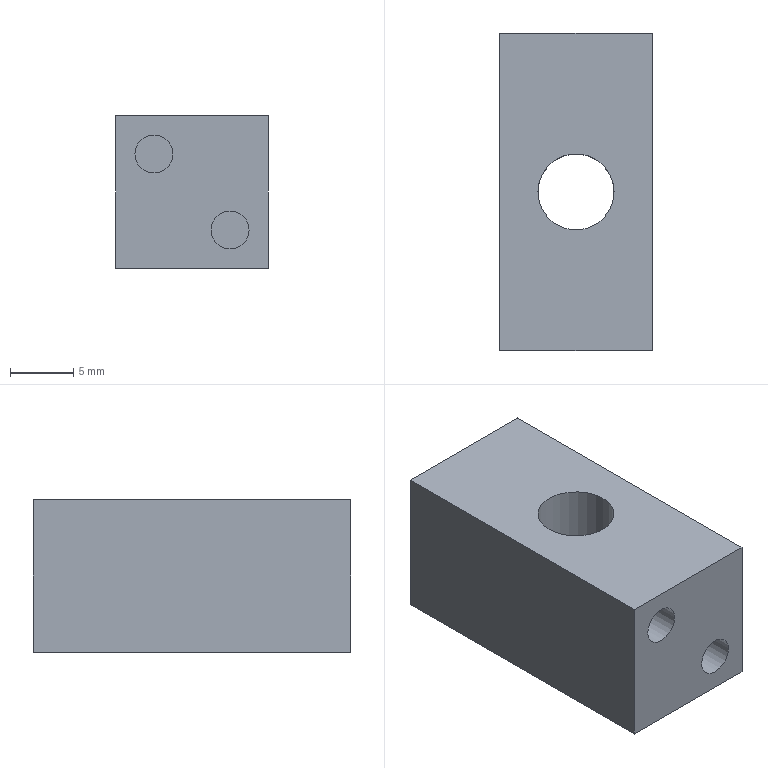Part | STEP file | 1-53.5 | 1 solid | 15 faces | box 12 x 25 x 12 mm | volume 3063 mm3 | plane 10 | cylinder 5 | commonest cylinder face diameters 3 x4 6 x1
STEP:
#1=CARTESIAN_POINT('',(0.,0.,0.));
#2=DIRECTION('',(0.,0.,1.));
#3=DIRECTION('',(1.,0.,0.));
#4=AXIS2_PLACEMENT_3D('',#1,#2,#3);
#5=CARTESIAN_POINT('',(6.,12.5,-6.));
#6=VERTEX_POINT('',#5);
#7=CARTESIAN_POINT('',(6.,12.5,6.));
#8=VERTEX_POINT('',#7);
#9=CARTESIAN_POINT('',(6.,12.5,-6.));
#10=DIRECTION('',(0.,0.,1.));
#11=VECTOR('',#10,1.);
#12=LINE('',#9,#11);
#13=CARTESIAN_POINT('',(6.,0.,0.));
#14=DIRECTION('',(1.,0.,0.));
#15=DIRECTION('',(0.,0.,1.));
#16=AXIS2_PLACEMENT_3D('',#13,#14,#15);
#17=PLANE('',#16);
#18=CARTESIAN_POINT('',(-6.,-12.5));
#19=DIRECTION('',(1.,0.));
#20=VECTOR('',#19,1.);
#21=LINE('',#18,#20);
#22=(GEOMETRIC_REPRESENTATION_CONTEXT(2)PARAMETRIC_REPRESENTATION_CONTEXT()REPRESENTATION_CONTEXT('',''));
#23=DEFINITIONAL_REPRESENTATION('',(#21),#22);
#24=PCURVE('',#17,#23);
#25=CARTESIAN_POINT('',(0.,12.5,0.));
#26=DIRECTION('',(0.,-1.,0.));
#27=DIRECTION('',(1.,0.,0.));
#28=AXIS2_PLACEMENT_3D('',#25,#26,#27);
#29=PLANE('',#28);
#30=CARTESIAN_POINT('',(6.,-6.));
#31=DIRECTION('',(0.,1.));
#32=VECTOR('',#31,1.);
#33=LINE('',#30,#32);
#34=(GEOMETRIC_REPRESENTATION_CONTEXT(2)PARAMETRIC_REPRESENTATION_CONTEXT()REPRESENTATION_CONTEXT('',''));
#35=DEFINITIONAL_REPRESENTATION('',(#33),#34);
#36=PCURVE('',#29,#35);
#37=SURFACE_CURVE('',#12,(#24,#36),.PCURVE_S1.);
#38=EDGE_CURVE('',#6,#8,#37,.T.);
#39=ORIENTED_EDGE('',*,*,#38,.T.);
#40=CARTESIAN_POINT('',(6.,-12.5,6.));
#41=VERTEX_POINT('',#40);
#42=CARTESIAN_POINT('',(6.,12.5,6.));
#43=DIRECTION('',(0.,-1.,0.));
#44=VECTOR('',#43,1.);
#45=LINE('',#42,#44);
#46=CARTESIAN_POINT('',(6.,-12.5));
#47=DIRECTION('',(0.,1.));
#48=VECTOR('',#47,1.);
#49=LINE('',#46,#48);
#50=(GEOMETRIC_REPRESENTATION_CONTEXT(2)PARAMETRIC_REPRESENTATION_CONTEXT()REPRESENTATION_CONTEXT('',''));
#51=DEFINITIONAL_REPRESENTATION('',(#49),#50);
#52=PCURVE('',#17,#51);
#53=CARTESIAN_POINT('',(0.,0.,6.));
#54=DIRECTION('',(0.,0.,1.));
#55=DIRECTION('',(-1.,0.,0.));
#56=AXIS2_PLACEMENT_3D('',#53,#54,#55);
#57=PLANE('',#56);
#58=CARTESIAN_POINT('',(-6.,-12.5));
#59=DIRECTION('',(0.,1.));
#60=VECTOR('',#59,1.);
#61=LINE('',#58,#60);
#62=(GEOMETRIC_REPRESENTATION_CONTEXT(2)PARAMETRIC_REPRESENTATION_CONTEXT()REPRESENTATION_CONTEXT('',''));
#63=DEFINITIONAL_REPRESENTATION('',(#61),#62);
#64=PCURVE('',#57,#63);
#65=SURFACE_CURVE('',#45,(#52,#64),.PCURVE_S1.);
#66=EDGE_CURVE('',#8,#41,#65,.T.);
#67=ORIENTED_EDGE('',*,*,#66,.T.);
#68=CARTESIAN_POINT('',(6.,-12.5,-6.));
#69=VERTEX_POINT('',#68);
#70=CARTESIAN_POINT('',(6.,-12.5,-6.));
#71=DIRECTION('',(0.,0.,1.));
#72=VECTOR('',#71,1.);
#73=LINE('',#70,#72);
#74=CARTESIAN_POINT('',(-6.,12.5));
#75=DIRECTION('',(1.,0.));
#76=VECTOR('',#75,1.);
#77=LINE('',#74,#76);
#78=(GEOMETRIC_REPRESENTATION_CONTEXT(2)PARAMETRIC_REPRESENTATION_CONTEXT()REPRESENTATION_CONTEXT('',''));
#79=DEFINITIONAL_REPRESENTATION('',(#77),#78);
#80=PCURVE('',#17,#79);
#81=CARTESIAN_POINT('',(0.,-12.5,0.));
#82=DIRECTION('',(0.,-1.,0.));
#83=DIRECTION('',(1.,0.,0.));
#84=AXIS2_PLACEMENT_3D('',#81,#82,#83);
#85=PLANE('',#84);
#86=CARTESIAN_POINT('',(6.,-6.));
#87=DIRECTION('',(0.,1.));
#88=VECTOR('',#87,1.);
#89=LINE('',#86,#88);
#90=(GEOMETRIC_REPRESENTATION_CONTEXT(2)PARAMETRIC_REPRESENTATION_CONTEXT()REPRESENTATION_CONTEXT('',''));
#91=DEFINITIONAL_REPRESENTATION('',(#89),#90);
#92=PCURVE('',#85,#91);
#93=SURFACE_CURVE('',#73,(#80,#92),.PCURVE_S1.);
#94=EDGE_CURVE('',#69,#41,#93,.T.);
#95=ORIENTED_EDGE('',*,*,#94,.F.);
#96=CARTESIAN_POINT('',(6.,12.5,-6.));
#97=DIRECTION('',(0.,-1.,0.));
#98=VECTOR('',#97,1.);
#99=LINE('',#96,#98);
#100=CARTESIAN_POINT('',(-6.,-12.5));
#101=DIRECTION('',(0.,1.));
#102=VECTOR('',#101,1.);
#103=LINE('',#100,#102);
#104=(GEOMETRIC_REPRESENTATION_CONTEXT(2)PARAMETRIC_REPRESENTATION_CONTEXT()REPRESENTATION_CONTEXT('',''));
#105=DEFINITIONAL_REPRESENTATION('',(#103),#104);
#106=PCURVE('',#17,#105);
#107=CARTESIAN_POINT('',(0.,0.,-6.));
#108=DIRECTION('',(0.,0.,-1.));
#109=DIRECTION('',(1.,0.,0.));
#110=AXIS2_PLACEMENT_3D('',#107,#108,#109);
#111=PLANE('',#110);
#112=CARTESIAN_POINT('',(6.,-12.5));
#113=DIRECTION('',(0.,1.));
#114=VECTOR('',#113,1.);
#115=LINE('',#112,#114);
#116=(GEOMETRIC_REPRESENTATION_CONTEXT(2)PARAMETRIC_REPRESENTATION_CONTEXT()REPRESENTATION_CONTEXT('',''));
#117=DEFINITIONAL_REPRESENTATION('',(#115),#116);
#118=PCURVE('',#111,#117);
#119=SURFACE_CURVE('',#99,(#106,#118),.PCURVE_S1.);
#120=EDGE_CURVE('',#6,#69,#119,.T.);
#121=ORIENTED_EDGE('',*,*,#120,.F.);
#122=EDGE_LOOP('',(#39,#67,#95,#121));
#123=FACE_BOUND('',#122,.T.);
#124=ADVANCED_FACE('',(#123),#17,.T.);
#125=CARTESIAN_POINT('',(-6.,12.5,6.));
#126=VERTEX_POINT('',#125);
#127=CARTESIAN_POINT('',(-6.,12.5,-6.));
#128=VERTEX_POINT('',#127);
#129=CARTESIAN_POINT('',(-6.,12.5,6.));
#130=DIRECTION('',(0.,0.,-1.));
#131=VECTOR('',#130,1.);
#132=LINE('',#129,#131);
#133=CARTESIAN_POINT('',(-6.,0.,0.));
#134=DIRECTION('',(-1.,0.,0.));
#135=DIRECTION('',(0.,0.,-1.));
#136=AXIS2_PLACEMENT_3D('',#133,#134,#135);
#137=PLANE('',#136);
#138=CARTESIAN_POINT('',(-6.,-12.5));
#139=DIRECTION('',(1.,0.));
#140=VECTOR('',#139,1.);
#141=LINE('',#138,#140);
#142=(GEOMETRIC_REPRESENTATION_CONTEXT(2)PARAMETRIC_REPRESENTATION_CONTEXT()REPRESENTATION_CONTEXT('',''));
#143=DEFINITIONAL_REPRESENTATION('',(#141),#142);
#144=PCURVE('',#137,#143);
#145=CARTESIAN_POINT('',(-6.,6.));
#146=DIRECTION('',(0.,-1.));
#147=VECTOR('',#146,1.);
#148=LINE('',#145,#147);
#149=(GEOMETRIC_REPRESENTATION_CONTEXT(2)PARAMETRIC_REPRESENTATION_CONTEXT()REPRESENTATION_CONTEXT('',''));
#150=DEFINITIONAL_REPRESENTATION('',(#148),#149);
#151=PCURVE('',#29,#150);
#152=SURFACE_CURVE('',#132,(#144,#151),.PCURVE_S1.);
#153=EDGE_CURVE('',#126,#128,#152,.T.);
#154=ORIENTED_EDGE('',*,*,#153,.T.);
#155=CARTESIAN_POINT('',(-6.,-12.5,-6.));
#156=VERTEX_POINT('',#155);
#157=CARTESIAN_POINT('',(-6.,12.5,-6.));
#158=DIRECTION('',(0.,-1.,0.));
#159=VECTOR('',#158,1.);
#160=LINE('',#157,#159);
#161=CARTESIAN_POINT('',(6.,-12.5));
#162=DIRECTION('',(0.,1.));
#163=VECTOR('',#162,1.);
#164=LINE('',#161,#163);
#165=(GEOMETRIC_REPRESENTATION_CONTEXT(2)PARAMETRIC_REPRESENTATION_CONTEXT()REPRESENTATION_CONTEXT('',''));
#166=DEFINITIONAL_REPRESENTATION('',(#164),#165);
#167=PCURVE('',#137,#166);
#168=CARTESIAN_POINT('',(-6.,-12.5));
#169=DIRECTION('',(0.,1.));
#170=VECTOR('',#169,1.);
#171=LINE('',#168,#170);
#172=(GEOMETRIC_REPRESENTATION_CONTEXT(2)PARAMETRIC_REPRESENTATION_CONTEXT()REPRESENTATION_CONTEXT('',''));
#173=DEFINITIONAL_REPRESENTATION('',(#171),#172);
#174=PCURVE('',#111,#173);
#175=SURFACE_CURVE('',#160,(#167,#174),.PCURVE_S1.);
#176=EDGE_CURVE('',#128,#156,#175,.T.);
#177=ORIENTED_EDGE('',*,*,#176,.T.);
#178=CARTESIAN_POINT('',(-6.,-12.5,6.));
#179=VERTEX_POINT('',#178);
#180=CARTESIAN_POINT('',(-6.,-12.5,6.));
#181=DIRECTION('',(0.,0.,-1.));
#182=VECTOR('',#181,1.);
#183=LINE('',#180,#182);
#184=CARTESIAN_POINT('',(-6.,12.5));
#185=DIRECTION('',(1.,0.));
#186=VECTOR('',#185,1.);
#187=LINE('',#184,#186);
#188=(GEOMETRIC_REPRESENTATION_CONTEXT(2)PARAMETRIC_REPRESENTATION_CONTEXT()REPRESENTATION_CONTEXT('',''));
#189=DEFINITIONAL_REPRESENTATION('',(#187),#188);
#190=PCURVE('',#137,#189);
#191=CARTESIAN_POINT('',(-6.,6.));
#192=DIRECTION('',(0.,-1.));
#193=VECTOR('',#192,1.);
#194=LINE('',#191,#193);
#195=(GEOMETRIC_REPRESENTATION_CONTEXT(2)PARAMETRIC_REPRESENTATION_CONTEXT()REPRESENTATION_CONTEXT('',''));
#196=DEFINITIONAL_REPRESENTATION('',(#194),#195);
#197=PCURVE('',#85,#196);
#198=SURFACE_CURVE('',#183,(#190,#197),.PCURVE_S1.);
#199=EDGE_CURVE('',#179,#156,#198,.T.);
#200=ORIENTED_EDGE('',*,*,#199,.F.);
#201=CARTESIAN_POINT('',(-6.,12.5,6.));
#202=DIRECTION('',(0.,-1.,0.));
#203=VECTOR('',#202,1.);
#204=LINE('',#201,#203);
#205=CARTESIAN_POINT('',(-6.,-12.5));
#206=DIRECTION('',(0.,1.));
#207=VECTOR('',#206,1.);
#208=LINE('',#205,#207);
#209=(GEOMETRIC_REPRESENTATION_CONTEXT(2)PARAMETRIC_REPRESENTATION_CONTEXT()REPRESENTATION_CONTEXT('',''));
#210=DEFINITIONAL_REPRESENTATION('',(#208),#209);
#211=PCURVE('',#137,#210);
#212=CARTESIAN_POINT('',(6.,-12.5));
#213=DIRECTION('',(0.,1.));
#214=VECTOR('',#213,1.);
#215=LINE('',#212,#214);
#216=(GEOMETRIC_REPRESENTATION_CONTEXT(2)PARAMETRIC_REPRESENTATION_CONTEXT()REPRESENTATION_CONTEXT('',''));
#217=DEFINITIONAL_REPRESENTATION('',(#215),#216);
#218=PCURVE('',#57,#217);
#219=SURFACE_CURVE('',#204,(#211,#218),.PCURVE_S1.);
#220=EDGE_CURVE('',#126,#179,#219,.T.);
#221=ORIENTED_EDGE('',*,*,#220,.F.);
#222=EDGE_LOOP('',(#154,#177,#200,#221));
#223=FACE_BOUND('',#222,.T.);
#224=ADVANCED_FACE('',(#223),#137,.T.);
#225=CARTESIAN_POINT('',(-6.,-12.5,-6.));
#226=DIRECTION('',(1.,0.,0.));
#227=VECTOR('',#226,1.);
#228=LINE('',#225,#227);
#229=CARTESIAN_POINT('',(-6.,-6.));
#230=DIRECTION('',(1.,0.));
#231=VECTOR('',#230,1.);
#232=LINE('',#229,#231);
#233=(GEOMETRIC_REPRESENTATION_CONTEXT(2)PARAMETRIC_REPRESENTATION_CONTEXT()REPRESENTATION_CONTEXT('',''));
#234=DEFINITIONAL_REPRESENTATION('',(#232),#233);
#235=PCURVE('',#85,#234);
#236=CARTESIAN_POINT('',(-6.,12.5));
#237=DIRECTION('',(1.,0.));
#238=VECTOR('',#237,1.);
#239=LINE('',#236,#238);
#240=(GEOMETRIC_REPRESENTATION_CONTEXT(2)PARAMETRIC_REPRESENTATION_CONTEXT()REPRESENTATION_CONTEXT('',''));
#241=DEFINITIONAL_REPRESENTATION('',(#239),#240);
#242=PCURVE('',#111,#241);
#243=SURFACE_CURVE('',#228,(#235,#242),.PCURVE_S1.);
#244=EDGE_CURVE('',#156,#69,#243,.T.);
#245=ORIENTED_EDGE('',*,*,#244,.T.);
#246=ORIENTED_EDGE('',*,*,#94,.T.);
#247=CARTESIAN_POINT('',(6.,-12.5,6.));
#248=DIRECTION('',(-1.,0.,0.));
#249=VECTOR('',#248,1.);
#250=LINE('',#247,#249);
#251=CARTESIAN_POINT('',(6.,6.));
#252=DIRECTION('',(-1.,0.));
#253=VECTOR('',#252,1.);
#254=LINE('',#251,#253);
#255=(GEOMETRIC_REPRESENTATION_CONTEXT(2)PARAMETRIC_REPRESENTATION_CONTEXT()REPRESENTATION_CONTEXT('',''));
#256=DEFINITIONAL_REPRESENTATION('',(#254),#255);
#257=PCURVE('',#85,#256);
#258=CARTESIAN_POINT('',(-6.,12.5));
#259=DIRECTION('',(1.,0.));
#260=VECTOR('',#259,1.);
#261=LINE('',#258,#260);
#262=(GEOMETRIC_REPRESENTATION_CONTEXT(2)PARAMETRIC_REPRESENTATION_CONTEXT()REPRESENTATION_CONTEXT('',''));
#263=DEFINITIONAL_REPRESENTATION('',(#261),#262);
#264=PCURVE('',#57,#263);
#265=SURFACE_CURVE('',#250,(#257,#264),.PCURVE_S1.);
#266=EDGE_CURVE('',#41,#179,#265,.T.);
#267=ORIENTED_EDGE('',*,*,#266,.T.);
#268=ORIENTED_EDGE('',*,*,#199,.T.);
#269=EDGE_LOOP('',(#245,#246,#267,#268));
#270=FACE_BOUND('',#269,.T.);
#271=CARTESIAN_POINT('',(-1.5,-12.5,3.));
#272=VERTEX_POINT('',#271);
#273=CARTESIAN_POINT('',(-3.,-12.5,3.));
#274=DIRECTION('',(0.,-1.,0.));
#275=DIRECTION('',(1.,0.,0.));
#276=AXIS2_PLACEMENT_3D('',#273,#274,#275);
#277=CIRCLE('',#276,1.5);
#278=CARTESIAN_POINT('',(-3.,3.));
#279=DIRECTION('',(1.,0.));
#280=AXIS2_PLACEMENT_2D('',#278,#279);
#281=CIRCLE('',#280,1.5);
#282=(GEOMETRIC_REPRESENTATION_CONTEXT(2)PARAMETRIC_REPRESENTATION_CONTEXT()REPRESENTATION_CONTEXT('',''));
#283=DEFINITIONAL_REPRESENTATION('',(#281),#282);
#284=PCURVE('',#85,#283);
#285=CARTESIAN_POINT('',(-3.,-12.5,3.));
#286=DIRECTION('',(0.,1.,0.));
#287=DIRECTION('',(1.,0.,0.));
#288=AXIS2_PLACEMENT_3D('',#285,#286,#287);
#289=CYLINDRICAL_SURFACE('',#288,1.5);
#290=CARTESIAN_POINT('',(6.283,0.));
#291=DIRECTION('',(-1.,0.));
#292=VECTOR('',#291,1.);
#293=LINE('',#290,#292);
#294=(GEOMETRIC_REPRESENTATION_CONTEXT(2)PARAMETRIC_REPRESENTATION_CONTEXT()REPRESENTATION_CONTEXT('',''));
#295=DEFINITIONAL_REPRESENTATION('',(#293),#294);
#296=PCURVE('',#289,#295);
#297=SURFACE_CURVE('',#277,(#284,#296),.PCURVE_S1.);
#298=EDGE_CURVE('',#272,#272,#297,.T.);
#299=ORIENTED_EDGE('',*,*,#298,.F.);
#300=EDGE_LOOP('',(#299));
#301=FACE_BOUND('',#300,.T.);
#302=CARTESIAN_POINT('',(4.5,-12.5,-3.));
#303=VERTEX_POINT('',#302);
#304=CARTESIAN_POINT('',(3.,-12.5,-3.));
#305=DIRECTION('',(0.,-1.,0.));
#306=DIRECTION('',(1.,0.,0.));
#307=AXIS2_PLACEMENT_3D('',#304,#305,#306);
#308=CIRCLE('',#307,1.5);
#309=CARTESIAN_POINT('',(3.,-3.));
#310=DIRECTION('',(1.,0.));
#311=AXIS2_PLACEMENT_2D('',#309,#310);
#312=CIRCLE('',#311,1.5);
#313=(GEOMETRIC_REPRESENTATION_CONTEXT(2)PARAMETRIC_REPRESENTATION_CONTEXT()REPRESENTATION_CONTEXT('',''));
#314=DEFINITIONAL_REPRESENTATION('',(#312),#313);
#315=PCURVE('',#85,#314);
#316=CARTESIAN_POINT('',(3.,-12.5,-3.));
#317=DIRECTION('',(0.,1.,0.));
#318=DIRECTION('',(1.,0.,0.));
#319=AXIS2_PLACEMENT_3D('',#316,#317,#318);
#320=CYLINDRICAL_SURFACE('',#319,1.5);
#321=CARTESIAN_POINT('',(6.283,0.));
#322=DIRECTION('',(-1.,0.));
#323=VECTOR('',#322,1.);
#324=LINE('',#321,#323);
#325=(GEOMETRIC_REPRESENTATION_CONTEXT(2)PARAMETRIC_REPRESENTATION_CONTEXT()REPRESENTATION_CONTEXT('',''));
#326=DEFINITIONAL_REPRESENTATION('',(#324),#325);
#327=PCURVE('',#320,#326);
#328=SURFACE_CURVE('',#308,(#315,#327),.PCURVE_S1.);
#329=EDGE_CURVE('',#303,#303,#328,.T.);
#330=ORIENTED_EDGE('',*,*,#329,.F.);
#331=EDGE_LOOP('',(#330));
#332=FACE_BOUND('',#331,.T.);
#333=ADVANCED_FACE('',(#270,#301,#332),#85,.T.);
#334=CARTESIAN_POINT('',(-1.5,-5.5,3.));
#335=VERTEX_POINT('',#334);
#336=CARTESIAN_POINT('',(-1.5,-12.5,3.));
#337=DIRECTION('',(0.,1.,0.));
#338=VECTOR('',#337,1.);
#339=LINE('',#336,#338);
#340=CARTESIAN_POINT('',(6.283,0.));
#341=DIRECTION('',(0.,1.));
#342=VECTOR('',#341,1.);
#343=LINE('',#340,#342);
#344=(GEOMETRIC_REPRESENTATION_CONTEXT(2)PARAMETRIC_REPRESENTATION_CONTEXT()REPRESENTATION_CONTEXT('',''));
#345=DEFINITIONAL_REPRESENTATION('',(#343),#344);
#346=PCURVE('',#289,#345);
#347=CARTESIAN_POINT('',(0.,0.));
#348=DIRECTION('',(0.,1.));
#349=VECTOR('',#348,1.);
#350=LINE('',#347,#349);
#351=(GEOMETRIC_REPRESENTATION_CONTEXT(2)PARAMETRIC_REPRESENTATION_CONTEXT()REPRESENTATION_CONTEXT('',''));
#352=DEFINITIONAL_REPRESENTATION('',(#350),#351);
#353=PCURVE('',#289,#352);
#354=SEAM_CURVE('',#339,(#346,#353),.PCURVE_S1.);
#355=EDGE_CURVE('',#272,#335,#354,.T.);
#356=ORIENTED_EDGE('',*,*,#355,.T.);
#357=CARTESIAN_POINT('',(-3.,-5.5,3.));
#358=DIRECTION('',(0.,-1.,0.));
#359=DIRECTION('',(1.,0.,0.));
#360=AXIS2_PLACEMENT_3D('',#357,#358,#359);
#361=CIRCLE('',#360,1.5);
#362=CARTESIAN_POINT('',(6.283,7.));
#363=DIRECTION('',(-1.,0.));
#364=VECTOR('',#363,1.);
#365=LINE('',#362,#364);
#366=(GEOMETRIC_REPRESENTATION_CONTEXT(2)PARAMETRIC_REPRESENTATION_CONTEXT()REPRESENTATION_CONTEXT('',''));
#367=DEFINITIONAL_REPRESENTATION('',(#365),#366);
#368=PCURVE('',#289,#367);
#369=CARTESIAN_POINT('',(-3.402,-5.5,3.));
#370=DIRECTION('',(0.,-1.,0.));
#371=DIRECTION('',(1.,0.,0.));
#372=AXIS2_PLACEMENT_3D('',#369,#370,#371);
#373=PLANE('',#372);
#374=CARTESIAN_POINT('',(0.4019,0.));
#375=DIRECTION('',(1.,0.));
#376=AXIS2_PLACEMENT_2D('',#374,#375);
#377=CIRCLE('',#376,1.5);
#378=(GEOMETRIC_REPRESENTATION_CONTEXT(2)PARAMETRIC_REPRESENTATION_CONTEXT()REPRESENTATION_CONTEXT('',''));
#379=DEFINITIONAL_REPRESENTATION('',(#377),#378);
#380=PCURVE('',#373,#379);
#381=SURFACE_CURVE('',#361,(#368,#380),.PCURVE_S1.);
#382=EDGE_CURVE('',#335,#335,#381,.T.);
#383=ORIENTED_EDGE('',*,*,#382,.T.);
#384=ORIENTED_EDGE('',*,*,#355,.F.);
#385=ORIENTED_EDGE('',*,*,#298,.F.);
#386=EDGE_LOOP('',(#356,#383,#384,#385));
#387=FACE_BOUND('',#386,.F.);
#388=ADVANCED_FACE('',(#387),#289,.F.);
#389=CARTESIAN_POINT('',(4.5,-5.5,-3.));
#390=VERTEX_POINT('',#389);
#391=CARTESIAN_POINT('',(4.5,-12.5,-3.));
#392=DIRECTION('',(0.,1.,0.));
#393=VECTOR('',#392,1.);
#394=LINE('',#391,#393);
#395=CARTESIAN_POINT('',(6.283,0.));
#396=DIRECTION('',(0.,1.));
#397=VECTOR('',#396,1.);
#398=LINE('',#395,#397);
#399=(GEOMETRIC_REPRESENTATION_CONTEXT(2)PARAMETRIC_REPRESENTATION_CONTEXT()REPRESENTATION_CONTEXT('',''));
#400=DEFINITIONAL_REPRESENTATION('',(#398),#399);
#401=PCURVE('',#320,#400);
#402=CARTESIAN_POINT('',(0.,0.));
#403=DIRECTION('',(0.,1.));
#404=VECTOR('',#403,1.);
#405=LINE('',#402,#404);
#406=(GEOMETRIC_REPRESENTATION_CONTEXT(2)PARAMETRIC_REPRESENTATION_CONTEXT()REPRESENTATION_CONTEXT('',''));
#407=DEFINITIONAL_REPRESENTATION('',(#405),#406);
#408=PCURVE('',#320,#407);
#409=SEAM_CURVE('',#394,(#401,#408),.PCURVE_S1.);
#410=EDGE_CURVE('',#303,#390,#409,.T.);
#411=ORIENTED_EDGE('',*,*,#410,.T.);
#412=CARTESIAN_POINT('',(3.,-5.5,-3.));
#413=DIRECTION('',(0.,-1.,0.));
#414=DIRECTION('',(1.,0.,0.));
#415=AXIS2_PLACEMENT_3D('',#412,#413,#414);
#416=CIRCLE('',#415,1.5);
#417=CARTESIAN_POINT('',(6.283,7.));
#418=DIRECTION('',(-1.,0.));
#419=VECTOR('',#418,1.);
#420=LINE('',#417,#419);
#421=(GEOMETRIC_REPRESENTATION_CONTEXT(2)PARAMETRIC_REPRESENTATION_CONTEXT()REPRESENTATION_CONTEXT('',''));
#422=DEFINITIONAL_REPRESENTATION('',(#420),#421);
#423=PCURVE('',#320,#422);
#424=CARTESIAN_POINT('',(2.598,-5.5,-3.));
#425=DIRECTION('',(0.,-1.,0.));
#426=DIRECTION('',(1.,0.,0.));
#427=AXIS2_PLACEMENT_3D('',#424,#425,#426);
#428=PLANE('',#427);
#429=CARTESIAN_POINT('',(0.4019,0.));
#430=DIRECTION('',(1.,0.));
#431=AXIS2_PLACEMENT_2D('',#429,#430);
#432=CIRCLE('',#431,1.5);
#433=(GEOMETRIC_REPRESENTATION_CONTEXT(2)PARAMETRIC_REPRESENTATION_CONTEXT()REPRESENTATION_CONTEXT('',''));
#434=DEFINITIONAL_REPRESENTATION('',(#432),#433);
#435=PCURVE('',#428,#434);
#436=SURFACE_CURVE('',#416,(#423,#435),.PCURVE_S1.);
#437=EDGE_CURVE('',#390,#390,#436,.T.);
#438=ORIENTED_EDGE('',*,*,#437,.T.);
#439=ORIENTED_EDGE('',*,*,#410,.F.);
#440=ORIENTED_EDGE('',*,*,#329,.F.);
#441=EDGE_LOOP('',(#411,#438,#439,#440));
#442=FACE_BOUND('',#441,.F.);
#443=ADVANCED_FACE('',(#442),#320,.F.);
#444=ORIENTED_EDGE('',*,*,#382,.T.);
#445=EDGE_LOOP('',(#444));
#446=FACE_BOUND('',#445,.T.);
#447=ADVANCED_FACE('',(#446),#373,.T.);
#448=ORIENTED_EDGE('',*,*,#437,.T.);
#449=EDGE_LOOP('',(#448));
#450=FACE_BOUND('',#449,.T.);
#451=ADVANCED_FACE('',(#450),#428,.T.);
#452=CARTESIAN_POINT('',(-6.,12.5,-6.));
#453=DIRECTION('',(1.,0.,0.));
#454=VECTOR('',#453,1.);
#455=LINE('',#452,#454);
#456=CARTESIAN_POINT('',(-6.,-12.5));
#457=DIRECTION('',(1.,0.));
#458=VECTOR('',#457,1.);
#459=LINE('',#456,#458);
#460=(GEOMETRIC_REPRESENTATION_CONTEXT(2)PARAMETRIC_REPRESENTATION_CONTEXT()REPRESENTATION_CONTEXT('',''));
#461=DEFINITIONAL_REPRESENTATION('',(#459),#460);
#462=PCURVE('',#111,#461);
#463=CARTESIAN_POINT('',(-6.,-6.));
#464=DIRECTION('',(1.,0.));
#465=VECTOR('',#464,1.);
#466=LINE('',#463,#465);
#467=(GEOMETRIC_REPRESENTATION_CONTEXT(2)PARAMETRIC_REPRESENTATION_CONTEXT()REPRESENTATION_CONTEXT('',''));
#468=DEFINITIONAL_REPRESENTATION('',(#466),#467);
#469=PCURVE('',#29,#468);
#470=SURFACE_CURVE('',#455,(#462,#469),.PCURVE_S1.);
#471=EDGE_CURVE('',#128,#6,#470,.T.);
#472=ORIENTED_EDGE('',*,*,#471,.T.);
#473=ORIENTED_EDGE('',*,*,#120,.T.);
#474=ORIENTED_EDGE('',*,*,#244,.F.);
#475=ORIENTED_EDGE('',*,*,#176,.F.);
#476=EDGE_LOOP('',(#472,#473,#474,#475));
#477=FACE_BOUND('',#476,.T.);
#478=CARTESIAN_POINT('',(3.,0.,-6.));
#479=VERTEX_POINT('',#478);
#480=CARTESIAN_POINT('',(0.,0.,-6.));
#481=DIRECTION('',(0.,0.,1.));
#482=DIRECTION('',(1.,0.,0.));
#483=AXIS2_PLACEMENT_3D('',#480,#481,#482);
#484=CIRCLE('',#483,3.);
#485=CARTESIAN_POINT('',(3.,0.));
#486=CARTESIAN_POINT('',(3.,-5.196));
#487=CARTESIAN_POINT('',(-1.5,-2.598));
#488=CARTESIAN_POINT('',(-6.,0.));
#489=CARTESIAN_POINT('',(-1.5,2.598));
#490=CARTESIAN_POINT('',(3.,5.196));
#491=CARTESIAN_POINT('',(3.,0.));
#492=(BOUNDED_CURVE()B_SPLINE_CURVE(2,(#485,#486,#487,#488,#489,#490,#491),.UNSPECIFIED.,.T.,.F.)B_SPLINE_CURVE_WITH_KNOTS((1,2,2,2,2,1),(-2.094,0.,2.094,4.189,6.283,8.378),.UNSPECIFIED.)CURVE()GEOMETRIC_REPRESENTATION_ITEM()RATIONAL_B_SPLINE_CURVE((1.,0.5,1.,0.5,1.,0.5,1.))REPRESENTATION_ITEM(''));
#493=(GEOMETRIC_REPRESENTATION_CONTEXT(2)PARAMETRIC_REPRESENTATION_CONTEXT()REPRESENTATION_CONTEXT('',''));
#494=DEFINITIONAL_REPRESENTATION('',(#492),#493);
#495=PCURVE('',#111,#494);
#496=CARTESIAN_POINT('',(0.,0.,6.));
#497=DIRECTION('',(0.,0.,-1.));
#498=DIRECTION('',(1.,0.,0.));
#499=AXIS2_PLACEMENT_3D('',#496,#497,#498);
#500=CYLINDRICAL_SURFACE('',#499,3.);
#501=CARTESIAN_POINT('',(6.283,12.));
#502=DIRECTION('',(-1.,0.));
#503=VECTOR('',#502,1.);
#504=LINE('',#501,#503);
#505=(GEOMETRIC_REPRESENTATION_CONTEXT(2)PARAMETRIC_REPRESENTATION_CONTEXT()REPRESENTATION_CONTEXT('',''));
#506=DEFINITIONAL_REPRESENTATION('',(#504),#505);
#507=PCURVE('',#500,#506);
#508=SURFACE_CURVE('',#484,(#495,#507),.PCURVE_S1.);
#509=EDGE_CURVE('',#479,#479,#508,.T.);
#510=ORIENTED_EDGE('',*,*,#509,.T.);
#511=EDGE_LOOP('',(#510));
#512=FACE_BOUND('',#511,.T.);
#513=ADVANCED_FACE('',(#477,#512),#111,.T.);
#514=CARTESIAN_POINT('',(6.,12.5,6.));
#515=DIRECTION('',(-1.,0.,0.));
#516=VECTOR('',#515,1.);
#517=LINE('',#514,#516);
#518=CARTESIAN_POINT('',(-6.,-12.5));
#519=DIRECTION('',(1.,0.));
#520=VECTOR('',#519,1.);
#521=LINE('',#518,#520);
#522=(GEOMETRIC_REPRESENTATION_CONTEXT(2)PARAMETRIC_REPRESENTATION_CONTEXT()REPRESENTATION_CONTEXT('',''));
#523=DEFINITIONAL_REPRESENTATION('',(#521),#522);
#524=PCURVE('',#57,#523);
#525=CARTESIAN_POINT('',(6.,6.));
#526=DIRECTION('',(-1.,0.));
#527=VECTOR('',#526,1.);
#528=LINE('',#525,#527);
#529=(GEOMETRIC_REPRESENTATION_CONTEXT(2)PARAMETRIC_REPRESENTATION_CONTEXT()REPRESENTATION_CONTEXT('',''));
#530=DEFINITIONAL_REPRESENTATION('',(#528),#529);
#531=PCURVE('',#29,#530);
#532=SURFACE_CURVE('',#517,(#524,#531),.PCURVE_S1.);
#533=EDGE_CURVE('',#8,#126,#532,.T.);
#534=ORIENTED_EDGE('',*,*,#533,.T.);
#535=ORIENTED_EDGE('',*,*,#220,.T.);
#536=ORIENTED_EDGE('',*,*,#266,.F.);
#537=ORIENTED_EDGE('',*,*,#66,.F.);
#538=EDGE_LOOP('',(#534,#535,#536,#537));
#539=FACE_BOUND('',#538,.T.);
#540=CARTESIAN_POINT('',(3.,0.,6.));
#541=VERTEX_POINT('',#540);
#542=CARTESIAN_POINT('',(0.,0.,6.));
#543=DIRECTION('',(0.,0.,1.));
#544=DIRECTION('',(1.,0.,0.));
#545=AXIS2_PLACEMENT_3D('',#542,#543,#544);
#546=CIRCLE('',#545,3.);
#547=CARTESIAN_POINT('',(0.,0.));
#548=DIRECTION('',(-1.,0.));
#549=AXIS2_PLACEMENT_2D('',#547,#548);
#550=CIRCLE('',#549,3.);
#551=(GEOMETRIC_REPRESENTATION_CONTEXT(2)PARAMETRIC_REPRESENTATION_CONTEXT()REPRESENTATION_CONTEXT('',''));
#552=DEFINITIONAL_REPRESENTATION('',(#550),#551);
#553=PCURVE('',#57,#552);
#554=CARTESIAN_POINT('',(6.283,0.));
#555=DIRECTION('',(-1.,0.));
#556=VECTOR('',#555,1.);
#557=LINE('',#554,#556);
#558=(GEOMETRIC_REPRESENTATION_CONTEXT(2)PARAMETRIC_REPRESENTATION_CONTEXT()REPRESENTATION_CONTEXT('',''));
#559=DEFINITIONAL_REPRESENTATION('',(#557),#558);
#560=PCURVE('',#500,#559);
#561=SURFACE_CURVE('',#546,(#553,#560),.PCURVE_S1.);
#562=EDGE_CURVE('',#541,#541,#561,.T.);
#563=ORIENTED_EDGE('',*,*,#562,.F.);
#564=EDGE_LOOP('',(#563));
#565=FACE_BOUND('',#564,.T.);
#566=ADVANCED_FACE('',(#539,#565),#57,.T.);
#567=CARTESIAN_POINT('',(3.,0.,6.));
#568=DIRECTION('',(0.,0.,-1.));
#569=VECTOR('',#568,1.);
#570=LINE('',#567,#569);
#571=CARTESIAN_POINT('',(6.283,0.));
#572=DIRECTION('',(0.,1.));
#573=VECTOR('',#572,1.);
#574=LINE('',#571,#573);
#575=(GEOMETRIC_REPRESENTATION_CONTEXT(2)PARAMETRIC_REPRESENTATION_CONTEXT()REPRESENTATION_CONTEXT('',''));
#576=DEFINITIONAL_REPRESENTATION('',(#574),#575);
#577=PCURVE('',#500,#576);
#578=CARTESIAN_POINT('',(0.,0.));
#579=DIRECTION('',(0.,1.));
#580=VECTOR('',#579,1.);
#581=LINE('',#578,#580);
#582=(GEOMETRIC_REPRESENTATION_CONTEXT(2)PARAMETRIC_REPRESENTATION_CONTEXT()REPRESENTATION_CONTEXT('',''));
#583=DEFINITIONAL_REPRESENTATION('',(#581),#582);
#584=PCURVE('',#500,#583);
#585=SEAM_CURVE('',#570,(#577,#584),.PCURVE_S1.);
#586=EDGE_CURVE('',#541,#479,#585,.T.);
#587=ORIENTED_EDGE('',*,*,#586,.T.);
#588=ORIENTED_EDGE('',*,*,#509,.T.);
#589=ORIENTED_EDGE('',*,*,#586,.F.);
#590=ORIENTED_EDGE('',*,*,#562,.F.);
#591=EDGE_LOOP('',(#587,#588,#589,#590));
#592=FACE_BOUND('',#591,.F.);
#593=ADVANCED_FACE('',(#592),#500,.F.);
#594=ORIENTED_EDGE('',*,*,#471,.T.);
#595=ORIENTED_EDGE('',*,*,#38,.T.);
#596=ORIENTED_EDGE('',*,*,#533,.T.);
#597=ORIENTED_EDGE('',*,*,#153,.T.);
#598=EDGE_LOOP('',(#594,#595,#596,#597));
#599=FACE_BOUND('',#598,.F.);
#600=CARTESIAN_POINT('',(-1.5,12.5,3.));
#601=VERTEX_POINT('',#600);
#602=CARTESIAN_POINT('',(-3.,12.5,3.));
#603=DIRECTION('',(0.,-1.,0.));
#604=DIRECTION('',(1.,0.,0.));
#605=AXIS2_PLACEMENT_3D('',#602,#603,#604);
#606=CIRCLE('',#605,1.5);
#607=CARTESIAN_POINT('',(-3.,3.));
#608=DIRECTION('',(1.,0.));
#609=AXIS2_PLACEMENT_2D('',#607,#608);
#610=CIRCLE('',#609,1.5);
#611=(GEOMETRIC_REPRESENTATION_CONTEXT(2)PARAMETRIC_REPRESENTATION_CONTEXT()REPRESENTATION_CONTEXT('',''));
#612=DEFINITIONAL_REPRESENTATION('',(#610),#611);
#613=PCURVE('',#29,#612);
#614=CARTESIAN_POINT('',(-3.,12.5,3.));
#615=DIRECTION('',(0.,-1.,0.));
#616=DIRECTION('',(1.,0.,0.));
#617=AXIS2_PLACEMENT_3D('',#614,#615,#616);
#618=CYLINDRICAL_SURFACE('',#617,1.5);
#619=CARTESIAN_POINT('',(0.,0.));
#620=DIRECTION('',(1.,0.));
#621=VECTOR('',#620,1.);
#622=LINE('',#619,#621);
#623=(GEOMETRIC_REPRESENTATION_CONTEXT(2)PARAMETRIC_REPRESENTATION_CONTEXT()REPRESENTATION_CONTEXT('',''));
#624=DEFINITIONAL_REPRESENTATION('',(#622),#623);
#625=PCURVE('',#618,#624);
#626=SURFACE_CURVE('',#606,(#613,#625),.PCURVE_S1.);
#627=EDGE_CURVE('',#601,#601,#626,.T.);
#628=ORIENTED_EDGE('',*,*,#627,.F.);
#629=EDGE_LOOP('',(#628));
#630=FACE_BOUND('',#629,.F.);
#631=CARTESIAN_POINT('',(4.5,12.5,-3.));
#632=VERTEX_POINT('',#631);
#633=CARTESIAN_POINT('',(3.,12.5,-3.));
#634=DIRECTION('',(0.,-1.,0.));
#635=DIRECTION('',(1.,0.,0.));
#636=AXIS2_PLACEMENT_3D('',#633,#634,#635);
#637=CIRCLE('',#636,1.5);
#638=CARTESIAN_POINT('',(3.,-3.));
#639=DIRECTION('',(1.,0.));
#640=AXIS2_PLACEMENT_2D('',#638,#639);
#641=CIRCLE('',#640,1.5);
#642=(GEOMETRIC_REPRESENTATION_CONTEXT(2)PARAMETRIC_REPRESENTATION_CONTEXT()REPRESENTATION_CONTEXT('',''));
#643=DEFINITIONAL_REPRESENTATION('',(#641),#642);
#644=PCURVE('',#29,#643);
#645=CARTESIAN_POINT('',(3.,12.5,-3.));
#646=DIRECTION('',(0.,-1.,0.));
#647=DIRECTION('',(1.,0.,0.));
#648=AXIS2_PLACEMENT_3D('',#645,#646,#647);
#649=CYLINDRICAL_SURFACE('',#648,1.5);
#650=CARTESIAN_POINT('',(0.,0.));
#651=DIRECTION('',(1.,0.));
#652=VECTOR('',#651,1.);
#653=LINE('',#650,#652);
#654=(GEOMETRIC_REPRESENTATION_CONTEXT(2)PARAMETRIC_REPRESENTATION_CONTEXT()REPRESENTATION_CONTEXT('',''));
#655=DEFINITIONAL_REPRESENTATION('',(#653),#654);
#656=PCURVE('',#649,#655);
#657=SURFACE_CURVE('',#637,(#644,#656),.PCURVE_S1.);
#658=EDGE_CURVE('',#632,#632,#657,.T.);
#659=ORIENTED_EDGE('',*,*,#658,.F.);
#660=EDGE_LOOP('',(#659));
#661=FACE_BOUND('',#660,.F.);
#662=ADVANCED_FACE('',(#599,#630,#661),#29,.F.);
#663=ORIENTED_EDGE('',*,*,#627,.T.);
#664=CARTESIAN_POINT('',(-1.5,5.5,3.));
#665=VERTEX_POINT('',#664);
#666=CARTESIAN_POINT('',(-1.5,12.5,3.));
#667=DIRECTION('',(0.,-1.,0.));
#668=VECTOR('',#667,1.);
#669=LINE('',#666,#668);
#670=CARTESIAN_POINT('',(6.283,0.));
#671=DIRECTION('',(0.,1.));
#672=VECTOR('',#671,1.);
#673=LINE('',#670,#672);
#674=(GEOMETRIC_REPRESENTATION_CONTEXT(2)PARAMETRIC_REPRESENTATION_CONTEXT()REPRESENTATION_CONTEXT('',''));
#675=DEFINITIONAL_REPRESENTATION('',(#673),#674);
#676=PCURVE('',#618,#675);
#677=CARTESIAN_POINT('',(0.,0.));
#678=DIRECTION('',(0.,1.));
#679=VECTOR('',#678,1.);
#680=LINE('',#677,#679);
#681=(GEOMETRIC_REPRESENTATION_CONTEXT(2)PARAMETRIC_REPRESENTATION_CONTEXT()REPRESENTATION_CONTEXT('',''));
#682=DEFINITIONAL_REPRESENTATION('',(#680),#681);
#683=PCURVE('',#618,#682);
#684=SEAM_CURVE('',#669,(#676,#683),.PCURVE_S1.);
#685=EDGE_CURVE('',#601,#665,#684,.T.);
#686=ORIENTED_EDGE('',*,*,#685,.T.);
#687=CARTESIAN_POINT('',(-3.,5.5,3.));
#688=DIRECTION('',(0.,-1.,0.));
#689=DIRECTION('',(1.,0.,0.));
#690=AXIS2_PLACEMENT_3D('',#687,#688,#689);
#691=CIRCLE('',#690,1.5);
#692=CARTESIAN_POINT('',(0.,7.));
#693=DIRECTION('',(1.,0.));
#694=VECTOR('',#693,1.);
#695=LINE('',#692,#694);
#696=(GEOMETRIC_REPRESENTATION_CONTEXT(2)PARAMETRIC_REPRESENTATION_CONTEXT()REPRESENTATION_CONTEXT('',''));
#697=DEFINITIONAL_REPRESENTATION('',(#695),#696);
#698=PCURVE('',#618,#697);
#699=CARTESIAN_POINT('',(-3.402,5.5,3.));
#700=DIRECTION('',(0.,-1.,0.));
#701=DIRECTION('',(1.,0.,0.));
#702=AXIS2_PLACEMENT_3D('',#699,#700,#701);
#703=PLANE('',#702);
#704=CARTESIAN_POINT('',(0.4019,0.));
#705=DIRECTION('',(1.,0.));
#706=AXIS2_PLACEMENT_2D('',#704,#705);
#707=CIRCLE('',#706,1.5);
#708=(GEOMETRIC_REPRESENTATION_CONTEXT(2)PARAMETRIC_REPRESENTATION_CONTEXT()REPRESENTATION_CONTEXT('',''));
#709=DEFINITIONAL_REPRESENTATION('',(#707),#708);
#710=PCURVE('',#703,#709);
#711=SURFACE_CURVE('',#691,(#698,#710),.PCURVE_S1.);
#712=EDGE_CURVE('',#665,#665,#711,.T.);
#713=ORIENTED_EDGE('',*,*,#712,.F.);
#714=ORIENTED_EDGE('',*,*,#685,.F.);
#715=EDGE_LOOP('',(#663,#686,#713,#714));
#716=FACE_BOUND('',#715,.F.);
#717=ADVANCED_FACE('',(#716),#618,.F.);
#718=ORIENTED_EDGE('',*,*,#658,.T.);
#719=CARTESIAN_POINT('',(4.5,5.5,-3.));
#720=VERTEX_POINT('',#719);
#721=CARTESIAN_POINT('',(4.5,12.5,-3.));
#722=DIRECTION('',(0.,-1.,0.));
#723=VECTOR('',#722,1.);
#724=LINE('',#721,#723);
#725=CARTESIAN_POINT('',(6.283,0.));
#726=DIRECTION('',(0.,1.));
#727=VECTOR('',#726,1.);
#728=LINE('',#725,#727);
#729=(GEOMETRIC_REPRESENTATION_CONTEXT(2)PARAMETRIC_REPRESENTATION_CONTEXT()REPRESENTATION_CONTEXT('',''));
#730=DEFINITIONAL_REPRESENTATION('',(#728),#729);
#731=PCURVE('',#649,#730);
#732=CARTESIAN_POINT('',(0.,0.));
#733=DIRECTION('',(0.,1.));
#734=VECTOR('',#733,1.);
#735=LINE('',#732,#734);
#736=(GEOMETRIC_REPRESENTATION_CONTEXT(2)PARAMETRIC_REPRESENTATION_CONTEXT()REPRESENTATION_CONTEXT('',''));
#737=DEFINITIONAL_REPRESENTATION('',(#735),#736);
#738=PCURVE('',#649,#737);
#739=SEAM_CURVE('',#724,(#731,#738),.PCURVE_S1.);
#740=EDGE_CURVE('',#632,#720,#739,.T.);
#741=ORIENTED_EDGE('',*,*,#740,.T.);
#742=CARTESIAN_POINT('',(3.,5.5,-3.));
#743=DIRECTION('',(0.,-1.,0.));
#744=DIRECTION('',(1.,0.,0.));
#745=AXIS2_PLACEMENT_3D('',#742,#743,#744);
#746=CIRCLE('',#745,1.5);
#747=CARTESIAN_POINT('',(0.,7.));
#748=DIRECTION('',(1.,0.));
#749=VECTOR('',#748,1.);
#750=LINE('',#747,#749);
#751=(GEOMETRIC_REPRESENTATION_CONTEXT(2)PARAMETRIC_REPRESENTATION_CONTEXT()REPRESENTATION_CONTEXT('',''));
#752=DEFINITIONAL_REPRESENTATION('',(#750),#751);
#753=PCURVE('',#649,#752);
#754=CARTESIAN_POINT('',(2.598,5.5,-3.));
#755=DIRECTION('',(0.,-1.,0.));
#756=DIRECTION('',(1.,0.,0.));
#757=AXIS2_PLACEMENT_3D('',#754,#755,#756);
#758=PLANE('',#757);
#759=CARTESIAN_POINT('',(0.4019,0.));
#760=DIRECTION('',(1.,0.));
#761=AXIS2_PLACEMENT_2D('',#759,#760);
#762=CIRCLE('',#761,1.5);
#763=(GEOMETRIC_REPRESENTATION_CONTEXT(2)PARAMETRIC_REPRESENTATION_CONTEXT()REPRESENTATION_CONTEXT('',''));
#764=DEFINITIONAL_REPRESENTATION('',(#762),#763);
#765=PCURVE('',#758,#764);
#766=SURFACE_CURVE('',#746,(#753,#765),.PCURVE_S1.);
#767=EDGE_CURVE('',#720,#720,#766,.T.);
#768=ORIENTED_EDGE('',*,*,#767,.F.);
#769=ORIENTED_EDGE('',*,*,#740,.F.);
#770=EDGE_LOOP('',(#718,#741,#768,#769));
#771=FACE_BOUND('',#770,.F.);
#772=ADVANCED_FACE('',(#771),#649,.F.);
#773=ORIENTED_EDGE('',*,*,#712,.T.);
#774=EDGE_LOOP('',(#773));
#775=FACE_BOUND('',#774,.F.);
#776=ADVANCED_FACE('',(#775),#703,.F.);
#777=ORIENTED_EDGE('',*,*,#767,.T.);
#778=EDGE_LOOP('',(#777));
#779=FACE_BOUND('',#778,.F.);
#780=ADVANCED_FACE('',(#779),#758,.F.);
#781=CLOSED_SHELL('',(#124,#224,#333,#388,#443,#447,#451,#513,#566,#593,#662,#717,#772,#776,#780));
#782=MANIFOLD_SOLID_BREP('',#781);
#783=(LENGTH_UNIT()NAMED_UNIT(*)SI_UNIT(.MILLI.,.METRE.));
#784=UNCERTAINTY_MEASURE_WITH_UNIT(LENGTH_MEASURE(0.0000001),#783,'','');
#785=(NAMED_UNIT(*)PLANE_ANGLE_UNIT()SI_UNIT($,.RADIAN.));
#786=(NAMED_UNIT(*)SI_UNIT($,.STERADIAN.)SOLID_ANGLE_UNIT());
#787=(GEOMETRIC_REPRESENTATION_CONTEXT(3)GLOBAL_UNCERTAINTY_ASSIGNED_CONTEXT((#784))GLOBAL_UNIT_ASSIGNED_CONTEXT((#783,#785,#786))REPRESENTATION_CONTEXT('',''));
#788=ADVANCED_BREP_SHAPE_REPRESENTATION('',(#4,#782),#787);